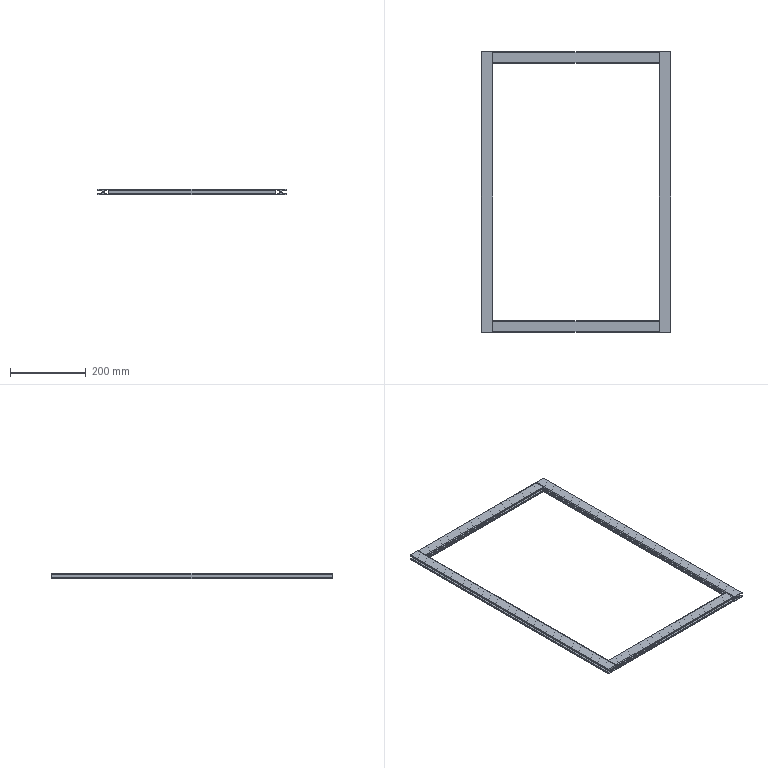Part | STEP file | 001-002-Door frame_default<machined> | 4 solids | 144 faces | box 498 x 738 x 15 mm | volume 556092 mm3 | plane 120 | cylinder 24 | commonest cylinder face diameters 3 x16 5 x8